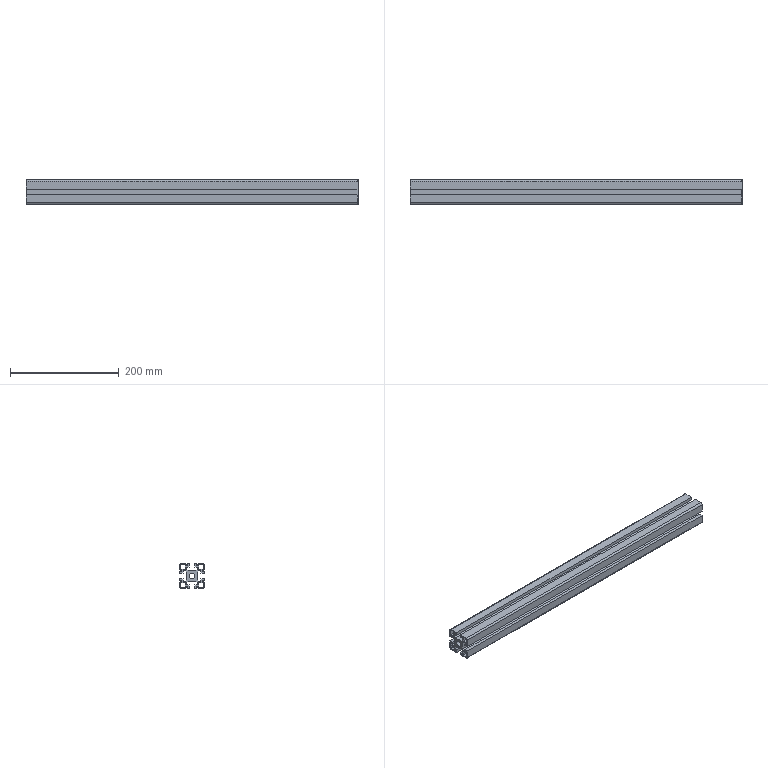Part | STEP file | bosch_3842990520_3kqsoefwhpgbs6igd9j6s2bp3 | 1 solid | 87 faces | box 610 x 45 x 45 mm | volume 498823 mm3 | plane 78 | cylinder 9 | commonest cylinder face diameters 2 x4 6 x4 10 x1